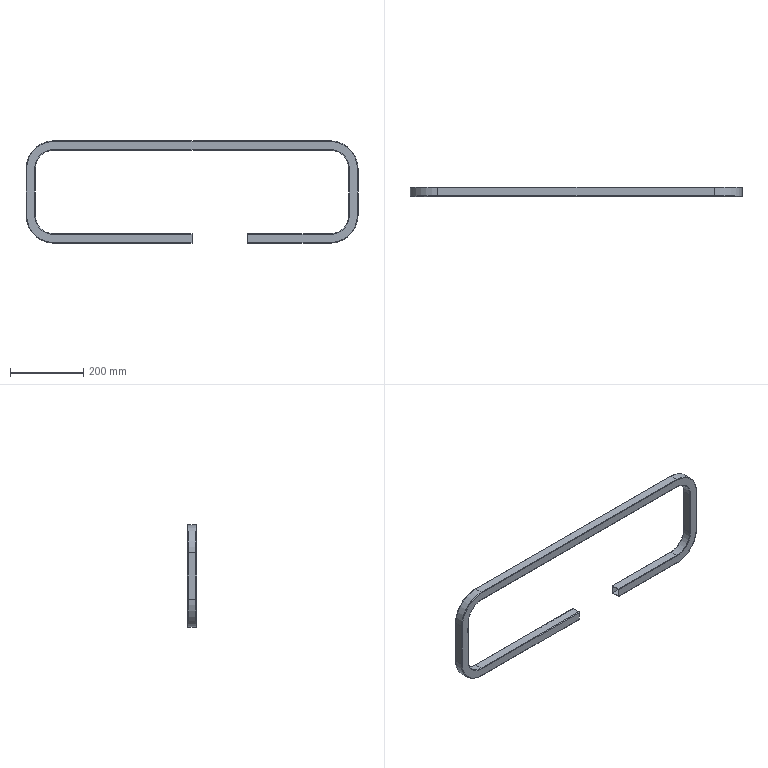Part | NX | features BREP 1 | 1 solid | 78 faces | box 906.78 x 25.4 x 279.4 mm | volume 368566 mm3 | cylinder 36 | plane 26 | torus 16 | commonest cylinder face diameters 3.175 x20 101.6 x4 105.562 x4 148.438 x4 152.4 x4